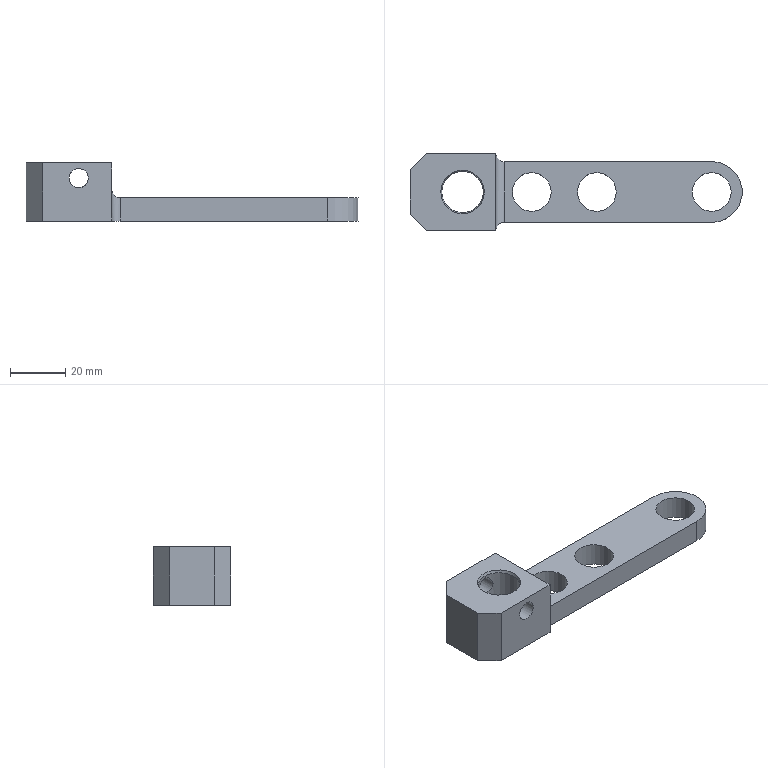NC program | NX | posted with a generic post | part box 120 x 28 x 21 mm
Whole program:
N10 G17 G21 G94 G90
(DRILLING_3_COPY , TOOL : 倒角D6-90度)
N12 T03 M6
N14 G54
N16 G17 G0 G90 X-19.008 Y15.5 B0. C0. S1200 M3
N18 G43 Z20. H3
N20 G94 G81 G99 Z-1. B-180. F60. R3.
N22 G80
N24 G0 X-19.008 Y15.5 Z20.
N26 M5
(DRILLING_4_COPY , TOOL : 钻头D6.8-73-105)
N28 T09 M6
N30 G54
N32 G17 G0 G90 X-19.008 Y15.5 B0. C0. S800 M3
N34 G43 Z20. H9
N36 G94 G81 G99 Z-10. B-180. F60. R3.
N38 G80
N40 G0 X-19.008 Y15.5 Z20.
N42 M5
(PLANAR_MILL_5_COPY_COPY_COPY , TOOL : 倒角D6-90度)
N44 T03 M6
N46 G54
N48 G17 G0 G90 X-19.273 Y14.432 B0. C0. S3000 M3
N50 G43 Z20. H3
N52 Z0. B-180.
N54 G94 G1 Z-2. F60.
N56 G41 X-19.308 Y14.235 D3
N58 Y14.2
N60 G3 X-19.008 Y13.9 R0.3
N62 X-17.408 Y15.5 R1.6
N64 X-19.008 Y13.9 R-1.6
N66 X-18.708 Y14.2 R0.3
N68 G1 Y14.235
N70 G40
N72 X-18.742 Y14.432
N74 Z0.
N76 G0 Z20.
N78 M5
(PLANAR_MILL_5_COPY_1 , TOOL : D6-18-D6-50-3T-精)
N80 T06 M6
N82 G54
N84 G17 G0 G90 X-19.087 Y15.478 B0. C0. S3000 M3
N86 G43 Z20. H6
N88 Z-7. B-180.
N90 G94 G1 Z-9. F60.
N92 G41 X-19.308 Y15.418 D6
N94 G3 X-19.008 Y15.118 R0.3
N96 X-18.626 Y15.5 R0.382
N98 X-19.008 Y15.118 R-0.382
N100 X-18.708 Y15.418 R0.3
N102 G40
N104 G1 X-18.725 Y15.516
N106 X-19.29 Y15.51
N108 G41 X-19.308 Y15.412
N110 G3 X-19.008 Y15.112 R0.3
N112 X-18.62 Y15.5 R0.388
N114 X-19.008 Y15.112 R-0.388
N116 X-18.708 Y15.412 R0.3
N118 G40
N120 G1 X-18.725 Y15.51
N122 X-19.29 Y15.504
N124 G41 X-19.308 Y15.406
N126 G3 X-19.008 Y15.106 R0.3
N128 X-18.614 Y15.5 R0.394
N130 X-19.008 Y15.106 R-0.394
N132 X-18.708 Y15.406 R0.3
N134 G40
N136 G1 X-18.725 Y15.504
N138 X-19.29 Y15.498
N140 G41 X-19.308 Y15.4
N142 G3 X-19.008 Y15.1 R0.3
N144 X-18.608 Y15.5 R0.4
N146 X-19.008 Y15.1 R-0.4
N148 X-18.708 Y15.4 R0.3
N150 G40
N152 G1 X-18.913 Y15.468
N154 Z-7.
N156 G0 Z20.
(PLANAR_MILL_5_COPY_COPY_1 , TOOL : D6-18-D6-50-3T-精)
N158 X-18.991 Y15.469
N160 Z-7.
N162 G1 Z-9. F30.
N164 G41 X-19.174 Y15.389
N166 X-19.308 Y15.3
N168 G3 X-19.008 Y15. R0.3
N170 X-18.508 Y15.5 R0.5
N172 X-19.008 Y15. R-0.5
N174 X-18.708 Y15.3 R0.3
N176 G40
N178 G1 X-18.742 Y15.497
N180 X-19.273
N182 G41 X-19.308 Y15.3
N184 G3 X-19.008 Y15. R0.3
N186 X-18.508 Y15.5 R0.5
N188 X-19.008 Y15. R-0.5
N190 X-18.708 Y15.3 R0.3
N192 G40
N194 G1 X-18.742 Y15.497
N196 X-19.273
N198 G41 X-19.308 Y15.3
N200 G3 X-19.008 Y15. R0.3
N202 X-18.508 Y15.5 R0.5
N204 X-19.008 Y15. R-0.5
N206 X-18.708 Y15.3 R0.3
N208 G1 X-18.841 Y15.389
N210 G40
N212 X-19.024 Y15.469
N214 Z-7.
N216 G0 Z20.
N218 M5
N220 M2